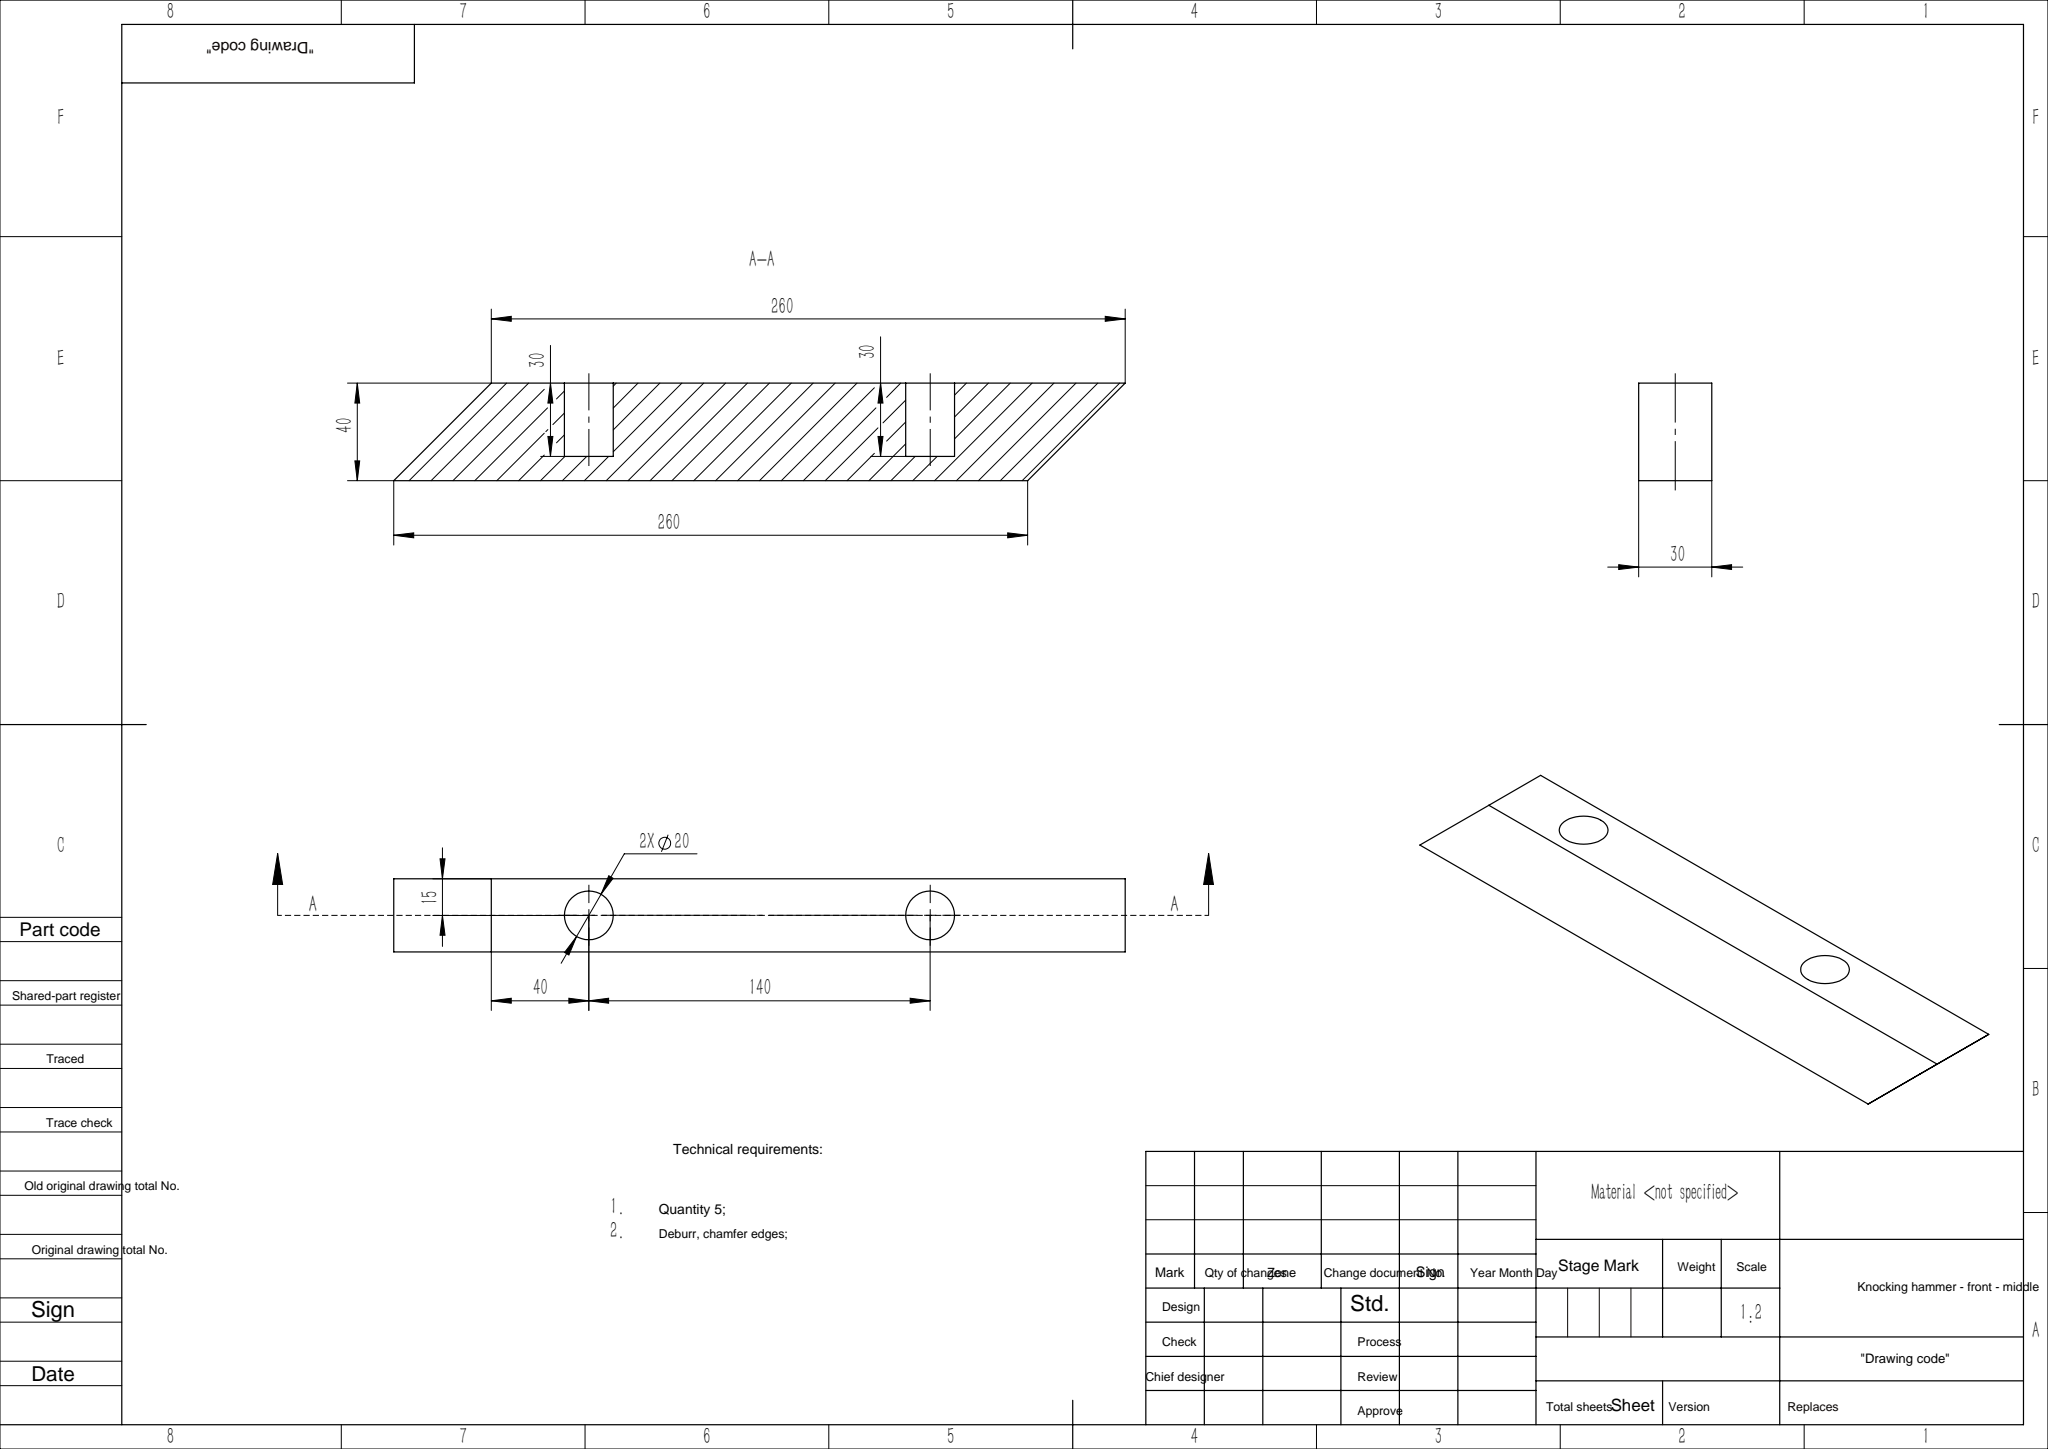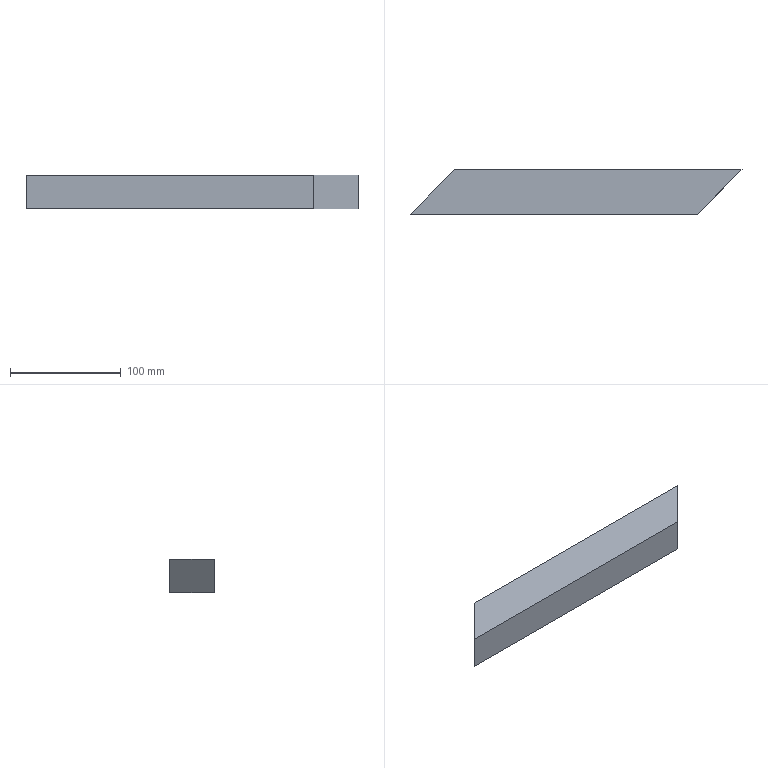Part | SolidWorks | features ICE 5, Extrusion 1 | 1 solid | 12 faces | box 300 x 40 x 30 mm | volume 293150 mm3 | plane 8 | cylinder 4 | commonest cylinder face diameters 20 x4
STEP:
#1=CARTESIAN_POINT('',(-70.,10.,-10.));
#2=VERTEX_POINT('',#1);
#3=CARTESIAN_POINT('',(-70.,10.,10.));
#4=VERTEX_POINT('',#3);
#5=CARTESIAN_POINT('',(-70.,10.,0.));
#6=DIRECTION('',(0.,1.,0.));
#7=DIRECTION('',(0.,0.,-1.));
#8=AXIS2_PLACEMENT_3D('',#5,#6,#7);
#9=CIRCLE('',#8,10.);
#10=EDGE_CURVE('',#2,#4,#9,.T.);
#11=ORIENTED_EDGE('',*,*,#10,.F.);
#12=CARTESIAN_POINT('',(-70.,40.,-10.));
#13=VERTEX_POINT('',#12);
#14=CARTESIAN_POINT('',(-70.,10.,-10.));
#15=DIRECTION('',(0.,1.,0.));
#16=VECTOR('',#15,1000.);
#17=LINE('',#14,#16);
#18=EDGE_CURVE('',#2,#13,#17,.T.);
#19=ORIENTED_EDGE('',*,*,#18,.T.);
#20=CARTESIAN_POINT('',(-70.,40.,10.));
#21=VERTEX_POINT('',#20);
#22=CARTESIAN_POINT('',(-70.,40.,0.));
#23=DIRECTION('',(0.,1.,0.));
#24=DIRECTION('',(0.,0.,-1.));
#25=AXIS2_PLACEMENT_3D('',#22,#23,#24);
#26=CIRCLE('',#25,10.);
#27=EDGE_CURVE('',#13,#21,#26,.T.);
#28=ORIENTED_EDGE('',*,*,#27,.T.);
#29=CARTESIAN_POINT('',(-70.,10.,10.));
#30=DIRECTION('',(0.,1.,0.));
#31=VECTOR('',#30,1000.);
#32=LINE('',#29,#31);
#33=EDGE_CURVE('',#4,#21,#32,.T.);
#34=ORIENTED_EDGE('',*,*,#33,.F.);
#35=EDGE_LOOP('',(#11,#19,#28,#34));
#36=FACE_OUTER_BOUND('',#35,.T.);
#37=CARTESIAN_POINT('',(-70.,10.,0.));
#38=DIRECTION('',(0.,1.,0.));
#39=DIRECTION('',(0.,0.,1.));
#40=AXIS2_PLACEMENT_3D('',#37,#38,#39);
#41=CYLINDRICAL_SURFACE('',#40,10.);
#42=ADVANCED_FACE('',(#36),#41,.F.);
#43=CARTESIAN_POINT('',(70.,10.,-10.));
#44=VERTEX_POINT('',#43);
#45=CARTESIAN_POINT('',(70.,10.,10.));
#46=VERTEX_POINT('',#45);
#47=CARTESIAN_POINT('',(70.,10.,0.));
#48=DIRECTION('',(0.,1.,0.));
#49=DIRECTION('',(0.,0.,1.));
#50=AXIS2_PLACEMENT_3D('',#47,#48,#49);
#51=CIRCLE('',#50,10.);
#52=EDGE_CURVE('',#44,#46,#51,.T.);
#53=ORIENTED_EDGE('',*,*,#52,.F.);
#54=CARTESIAN_POINT('',(70.,40.,-10.));
#55=VERTEX_POINT('',#54);
#56=CARTESIAN_POINT('',(70.,10.,-10.));
#57=DIRECTION('',(0.,1.,0.));
#58=VECTOR('',#57,1000.);
#59=LINE('',#56,#58);
#60=EDGE_CURVE('',#44,#55,#59,.T.);
#61=ORIENTED_EDGE('',*,*,#60,.T.);
#62=CARTESIAN_POINT('',(70.,40.,10.));
#63=VERTEX_POINT('',#62);
#64=CARTESIAN_POINT('',(70.,40.,0.));
#65=DIRECTION('',(0.,1.,0.));
#66=DIRECTION('',(0.,0.,1.));
#67=AXIS2_PLACEMENT_3D('',#64,#65,#66);
#68=CIRCLE('',#67,10.);
#69=EDGE_CURVE('',#55,#63,#68,.T.);
#70=ORIENTED_EDGE('',*,*,#69,.T.);
#71=CARTESIAN_POINT('',(70.,10.,10.));
#72=DIRECTION('',(0.,1.,0.));
#73=VECTOR('',#72,1000.);
#74=LINE('',#71,#73);
#75=EDGE_CURVE('',#46,#63,#74,.T.);
#76=ORIENTED_EDGE('',*,*,#75,.F.);
#77=EDGE_LOOP('',(#53,#61,#70,#76));
#78=FACE_OUTER_BOUND('',#77,.T.);
#79=CARTESIAN_POINT('',(70.,10.,0.));
#80=DIRECTION('',(0.,1.,0.));
#81=DIRECTION('',(0.,0.,1.));
#82=AXIS2_PLACEMENT_3D('',#79,#80,#81);
#83=CYLINDRICAL_SURFACE('',#82,10.);
#84=ADVANCED_FACE('',(#78),#83,.F.);
#85=CARTESIAN_POINT('',(110.,0.,-15.));
#86=VERTEX_POINT('',#85);
#87=CARTESIAN_POINT('',(-150.,0.,-15.));
#88=VERTEX_POINT('',#87);
#89=CARTESIAN_POINT('',(-135.,0.,-15.));
#90=DIRECTION('',(-1.,0.,0.));
#91=VECTOR('',#90,1000.);
#92=LINE('',#89,#91);
#93=EDGE_CURVE('',#86,#88,#92,.T.);
#94=ORIENTED_EDGE('',*,*,#93,.T.);
#95=CARTESIAN_POINT('',(-110.,40.,-15.));
#96=VERTEX_POINT('',#95);
#97=CARTESIAN_POINT('',(-150.,0.,-15.));
#98=DIRECTION('',(0.7071,0.7071,0.));
#99=VECTOR('',#98,1000.);
#100=LINE('',#97,#99);
#101=EDGE_CURVE('',#88,#96,#100,.T.);
#102=ORIENTED_EDGE('',*,*,#101,.T.);
#103=CARTESIAN_POINT('',(150.,40.,-15.));
#104=VERTEX_POINT('',#103);
#105=CARTESIAN_POINT('',(-135.,40.,-15.));
#106=DIRECTION('',(-1.,0.,0.));
#107=VECTOR('',#106,1000.);
#108=LINE('',#105,#107);
#109=EDGE_CURVE('',#104,#96,#108,.T.);
#110=ORIENTED_EDGE('',*,*,#109,.F.);
#111=CARTESIAN_POINT('',(150.,40.,-15.));
#112=DIRECTION('',(-0.7071,-0.7071,0.));
#113=VECTOR('',#112,1000.);
#114=LINE('',#111,#113);
#115=EDGE_CURVE('',#104,#86,#114,.T.);
#116=ORIENTED_EDGE('',*,*,#115,.T.);
#117=EDGE_LOOP('',(#94,#102,#110,#116));
#118=FACE_OUTER_BOUND('',#117,.T.);
#119=CARTESIAN_POINT('',(-135.,40.,-15.));
#120=DIRECTION('',(0.,0.,1.));
#121=DIRECTION('',(1.,0.,0.));
#122=AXIS2_PLACEMENT_3D('',#119,#120,#121);
#123=PLANE('',#122);
#124=ADVANCED_FACE('',(#118),#123,.F.);
#125=CARTESIAN_POINT('',(-110.,40.,15.));
#126=VERTEX_POINT('',#125);
#127=CARTESIAN_POINT('',(150.,40.,15.));
#128=VERTEX_POINT('',#127);
#129=CARTESIAN_POINT('',(-135.,40.,15.));
#130=DIRECTION('',(1.,0.,0.));
#131=VECTOR('',#130,1000.);
#132=LINE('',#129,#131);
#133=EDGE_CURVE('',#126,#128,#132,.T.);
#134=ORIENTED_EDGE('',*,*,#133,.F.);
#135=CARTESIAN_POINT('',(-150.,0.,15.));
#136=VERTEX_POINT('',#135);
#137=CARTESIAN_POINT('',(-150.,0.,15.));
#138=DIRECTION('',(0.7071,0.7071,0.));
#139=VECTOR('',#138,1000.);
#140=LINE('',#137,#139);
#141=EDGE_CURVE('',#136,#126,#140,.T.);
#142=ORIENTED_EDGE('',*,*,#141,.F.);
#143=CARTESIAN_POINT('',(110.,0.,15.));
#144=VERTEX_POINT('',#143);
#145=CARTESIAN_POINT('',(-135.,0.,15.));
#146=DIRECTION('',(1.,0.,0.));
#147=VECTOR('',#146,1000.);
#148=LINE('',#145,#147);
#149=EDGE_CURVE('',#136,#144,#148,.T.);
#150=ORIENTED_EDGE('',*,*,#149,.T.);
#151=CARTESIAN_POINT('',(150.,40.,15.));
#152=DIRECTION('',(-0.7071,-0.7071,0.));
#153=VECTOR('',#152,1000.);
#154=LINE('',#151,#153);
#155=EDGE_CURVE('',#128,#144,#154,.T.);
#156=ORIENTED_EDGE('',*,*,#155,.F.);
#157=EDGE_LOOP('',(#134,#142,#150,#156));
#158=FACE_OUTER_BOUND('',#157,.T.);
#159=CARTESIAN_POINT('',(-135.,40.,15.));
#160=DIRECTION('',(0.,0.,-1.));
#161=DIRECTION('',(-1.,0.,0.));
#162=AXIS2_PLACEMENT_3D('',#159,#160,#161);
#163=PLANE('',#162);
#164=ADVANCED_FACE('',(#158),#163,.F.);
#165=CARTESIAN_POINT('',(-70.,40.,0.));
#166=DIRECTION('',(0.,1.,0.));
#167=DIRECTION('',(0.,0.,-1.));
#168=AXIS2_PLACEMENT_3D('',#165,#166,#167);
#169=CIRCLE('',#168,10.);
#170=EDGE_CURVE('',#21,#13,#169,.T.);
#171=ORIENTED_EDGE('',*,*,#170,.F.);
#172=ORIENTED_EDGE('',*,*,#27,.F.);
#173=EDGE_LOOP('',(#171,#172));
#174=FACE_BOUND('',#173,.T.);
#175=CARTESIAN_POINT('',(70.,40.,0.));
#176=DIRECTION('',(0.,1.,0.));
#177=DIRECTION('',(0.,0.,1.));
#178=AXIS2_PLACEMENT_3D('',#175,#176,#177);
#179=CIRCLE('',#178,10.);
#180=EDGE_CURVE('',#63,#55,#179,.T.);
#181=ORIENTED_EDGE('',*,*,#180,.F.);
#182=ORIENTED_EDGE('',*,*,#69,.F.);
#183=EDGE_LOOP('',(#181,#182));
#184=FACE_BOUND('',#183,.T.);
#185=ORIENTED_EDGE('',*,*,#109,.T.);
#186=CARTESIAN_POINT('',(-110.,40.,-15.));
#187=DIRECTION('',(0.,0.,1.));
#188=VECTOR('',#187,1000.);
#189=LINE('',#186,#188);
#190=EDGE_CURVE('',#96,#126,#189,.T.);
#191=ORIENTED_EDGE('',*,*,#190,.T.);
#192=ORIENTED_EDGE('',*,*,#133,.T.);
#193=CARTESIAN_POINT('',(150.,40.,-15.));
#194=DIRECTION('',(0.,0.,1.));
#195=VECTOR('',#194,1000.);
#196=LINE('',#193,#195);
#197=EDGE_CURVE('',#104,#128,#196,.T.);
#198=ORIENTED_EDGE('',*,*,#197,.F.);
#199=EDGE_LOOP('',(#185,#191,#192,#198));
#200=FACE_OUTER_BOUND('',#199,.T.);
#201=CARTESIAN_POINT('',(0.,40.,0.));
#202=DIRECTION('',(0.,-1.,0.));
#203=DIRECTION('',(0.,0.,-1.));
#204=AXIS2_PLACEMENT_3D('',#201,#202,#203);
#205=PLANE('',#204);
#206=ADVANCED_FACE('',(#174,#184,#200),#205,.F.);
#207=CARTESIAN_POINT('',(110.,0.,-15.));
#208=DIRECTION('',(0.,0.,1.));
#209=VECTOR('',#208,1000.);
#210=LINE('',#207,#209);
#211=EDGE_CURVE('',#86,#144,#210,.T.);
#212=ORIENTED_EDGE('',*,*,#211,.T.);
#213=ORIENTED_EDGE('',*,*,#149,.F.);
#214=CARTESIAN_POINT('',(-150.,0.,-15.));
#215=DIRECTION('',(0.,0.,1.));
#216=VECTOR('',#215,1000.);
#217=LINE('',#214,#216);
#218=EDGE_CURVE('',#88,#136,#217,.T.);
#219=ORIENTED_EDGE('',*,*,#218,.F.);
#220=ORIENTED_EDGE('',*,*,#93,.F.);
#221=EDGE_LOOP('',(#212,#213,#219,#220));
#222=FACE_OUTER_BOUND('',#221,.T.);
#223=CARTESIAN_POINT('',(0.,0.,0.));
#224=DIRECTION('',(0.,-1.,0.));
#225=DIRECTION('',(0.,0.,-1.));
#226=AXIS2_PLACEMENT_3D('',#223,#224,#225);
#227=PLANE('',#226);
#228=ADVANCED_FACE('',(#222),#227,.T.);
#229=ORIENTED_EDGE('',*,*,#60,.F.);
#230=CARTESIAN_POINT('',(70.,10.,0.));
#231=DIRECTION('',(0.,1.,0.));
#232=DIRECTION('',(0.,0.,1.));
#233=AXIS2_PLACEMENT_3D('',#230,#231,#232);
#234=CIRCLE('',#233,10.);
#235=EDGE_CURVE('',#46,#44,#234,.T.);
#236=ORIENTED_EDGE('',*,*,#235,.F.);
#237=ORIENTED_EDGE('',*,*,#75,.T.);
#238=ORIENTED_EDGE('',*,*,#180,.T.);
#239=EDGE_LOOP('',(#229,#236,#237,#238));
#240=FACE_OUTER_BOUND('',#239,.T.);
#241=CARTESIAN_POINT('',(70.,10.,0.));
#242=DIRECTION('',(0.,1.,0.));
#243=DIRECTION('',(0.,0.,1.));
#244=AXIS2_PLACEMENT_3D('',#241,#242,#243);
#245=CYLINDRICAL_SURFACE('',#244,10.);
#246=ADVANCED_FACE('',(#240),#245,.F.);
#247=ORIENTED_EDGE('',*,*,#235,.T.);
#248=ORIENTED_EDGE('',*,*,#52,.T.);
#249=EDGE_LOOP('',(#247,#248));
#250=FACE_OUTER_BOUND('',#249,.T.);
#251=CARTESIAN_POINT('',(70.,10.,0.));
#252=DIRECTION('',(0.,1.,0.));
#253=DIRECTION('',(0.,0.,1.));
#254=AXIS2_PLACEMENT_3D('',#251,#252,#253);
#255=PLANE('',#254);
#256=ADVANCED_FACE('',(#250),#255,.T.);
#257=ORIENTED_EDGE('',*,*,#18,.F.);
#258=CARTESIAN_POINT('',(-70.,10.,0.));
#259=DIRECTION('',(0.,1.,0.));
#260=DIRECTION('',(0.,0.,-1.));
#261=AXIS2_PLACEMENT_3D('',#258,#259,#260);
#262=CIRCLE('',#261,10.);
#263=EDGE_CURVE('',#4,#2,#262,.T.);
#264=ORIENTED_EDGE('',*,*,#263,.F.);
#265=ORIENTED_EDGE('',*,*,#33,.T.);
#266=ORIENTED_EDGE('',*,*,#170,.T.);
#267=EDGE_LOOP('',(#257,#264,#265,#266));
#268=FACE_OUTER_BOUND('',#267,.T.);
#269=CARTESIAN_POINT('',(-70.,10.,0.));
#270=DIRECTION('',(0.,1.,0.));
#271=DIRECTION('',(0.,0.,1.));
#272=AXIS2_PLACEMENT_3D('',#269,#270,#271);
#273=CYLINDRICAL_SURFACE('',#272,10.);
#274=ADVANCED_FACE('',(#268),#273,.F.);
#275=ORIENTED_EDGE('',*,*,#263,.T.);
#276=ORIENTED_EDGE('',*,*,#10,.T.);
#277=EDGE_LOOP('',(#275,#276));
#278=FACE_OUTER_BOUND('',#277,.T.);
#279=CARTESIAN_POINT('',(-70.,10.,0.));
#280=DIRECTION('',(0.,-1.,0.));
#281=DIRECTION('',(0.,0.,-1.));
#282=AXIS2_PLACEMENT_3D('',#279,#280,#281);
#283=PLANE('',#282);
#284=ADVANCED_FACE('',(#278),#283,.F.);
#285=ORIENTED_EDGE('',*,*,#155,.T.);
#286=ORIENTED_EDGE('',*,*,#211,.F.);
#287=ORIENTED_EDGE('',*,*,#115,.F.);
#288=ORIENTED_EDGE('',*,*,#197,.T.);
#289=EDGE_LOOP('',(#285,#286,#287,#288));
#290=FACE_OUTER_BOUND('',#289,.T.);
#291=CARTESIAN_POINT('',(150.,40.,-15.));
#292=DIRECTION('',(-0.7071,0.7071,0.));
#293=DIRECTION('',(-0.7071,-0.7071,0.));
#294=AXIS2_PLACEMENT_3D('',#291,#292,#293);
#295=PLANE('',#294);
#296=ADVANCED_FACE('',(#290),#295,.F.);
#297=ORIENTED_EDGE('',*,*,#141,.T.);
#298=ORIENTED_EDGE('',*,*,#190,.F.);
#299=ORIENTED_EDGE('',*,*,#101,.F.);
#300=ORIENTED_EDGE('',*,*,#218,.T.);
#301=EDGE_LOOP('',(#297,#298,#299,#300));
#302=FACE_OUTER_BOUND('',#301,.T.);
#303=CARTESIAN_POINT('',(-150.,0.,-15.));
#304=DIRECTION('',(0.7071,-0.7071,0.));
#305=DIRECTION('',(0.7071,0.7071,0.));
#306=AXIS2_PLACEMENT_3D('',#303,#304,#305);
#307=PLANE('',#306);
#308=ADVANCED_FACE('',(#302),#307,.F.);
#309=CLOSED_SHELL('',(#42,#84,#124,#164,#206,#228,#246,#256,#274,#284,#296,#308));
#310=MANIFOLD_SOLID_BREP('',#309);
#311=CARTESIAN_POINT('',(0.,0.,0.));
#312=DIRECTION('',(0.,0.,1.));
#313=DIRECTION('',(1.,0.,0.));
#314=AXIS2_PLACEMENT_3D('',#311,#312,#313);
#315=(LENGTH_UNIT()NAMED_UNIT(*)SI_UNIT(.MILLI.,.METRE.));
#316=UNCERTAINTY_MEASURE_WITH_UNIT(LENGTH_MEASURE(0.00001),#315,'','');
#317=(NAMED_UNIT(*)PLANE_ANGLE_UNIT()SI_UNIT($,.RADIAN.));
#318=(NAMED_UNIT(*)SI_UNIT($,.STERADIAN.)SOLID_ANGLE_UNIT());
#319=(GEOMETRIC_REPRESENTATION_CONTEXT(3)GLOBAL_UNCERTAINTY_ASSIGNED_CONTEXT((#316))GLOBAL_UNIT_ASSIGNED_CONTEXT((#315,#317,#318))REPRESENTATION_CONTEXT('',''));
#320=ADVANCED_BREP_SHAPE_REPRESENTATION('',(#310,#314),#319);